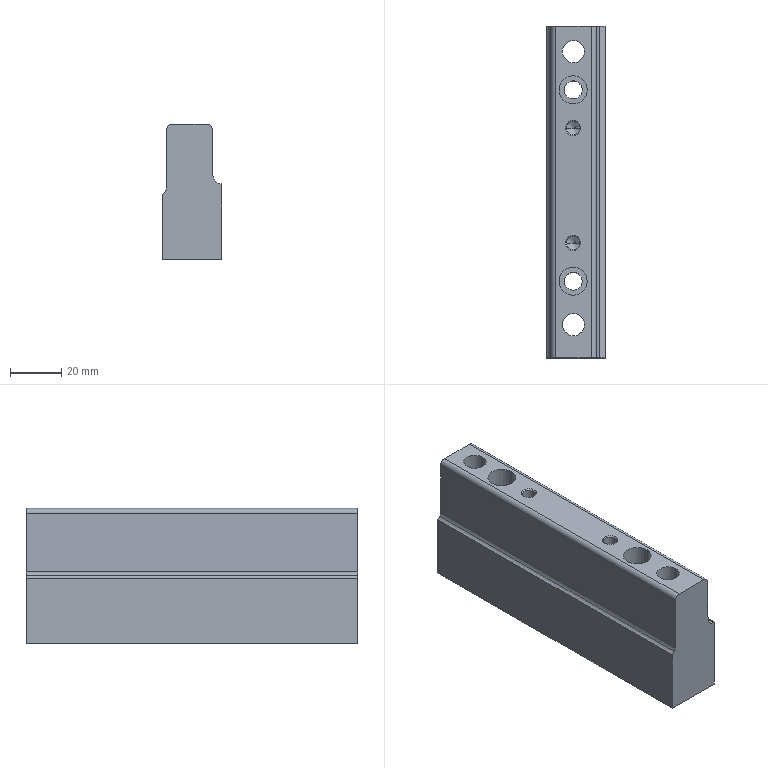Part | 1 solid | 48 faces | box 23.278 x 130 x 52.95 mm | volume 128778 mm3 | cylinder 27 | plane 13 | cone 8 | commonest cylinder face diameters 11 x8 5.2 x4 7 x4 8.8 x4 4 x2 6.648 x2